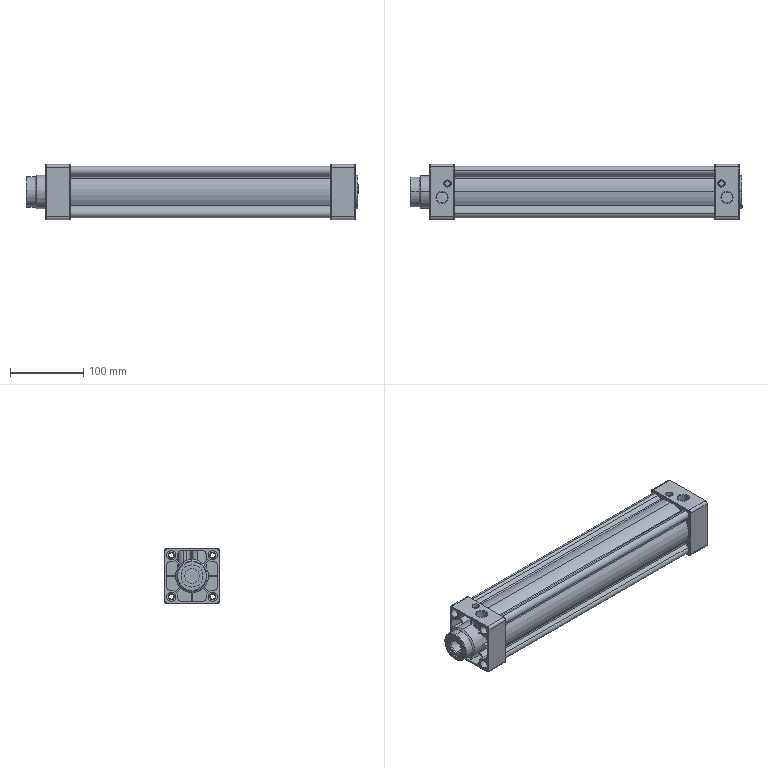Part | SolidWorks | features BaseBody 1 | 1 solid | 354 faces | box 452 x 75 x 75 mm | volume 612753 mm3 | cylinder 158 | plane 146 | cone 46 | spline 4 | commonest cylinder face diameters 12 x22 2.2 x18 8.7 x16 12.7 x16 7 x12 4 x10